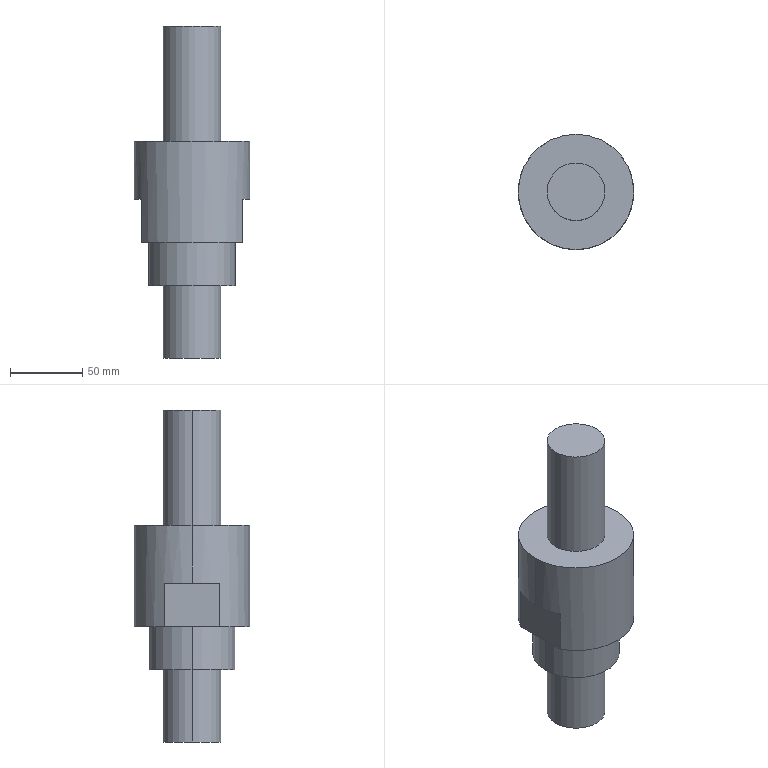Part | STEP file | Single sprocket shaft 2XG | 1 solid | 25 faces | box 80 x 80 x 230 mm | volume 591587 mm3 | cylinder 12 | plane 9 | cone 4 | commonest cylinder face diameters 5 x4 40 x4 60 x2 80 x2